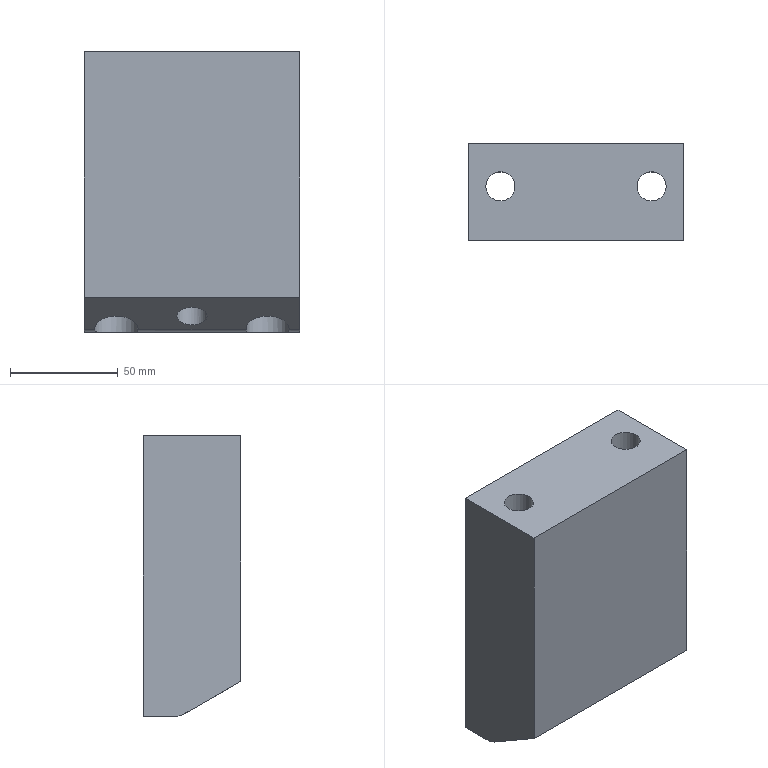Part | STEP file | lll_id3694_x_t | 1 solid | 20 faces | box 100 x 45 x 130 mm | volume 491265 mm3 | plane 10 | cylinder 9 | cone 1 | commonest cylinder face diameters 20 x3 13.509 x2 20.008 x2 10.505 x1 14 x1
STEP:
#1=CARTESIAN_POINT('',(2964.747,-53.5,17.5));
#2=VERTEX_POINT('',#1);
#3=CARTESIAN_POINT('',(2970.,-53.5,17.5));
#4=DIRECTION('',(0.,0.,-1.));
#5=DIRECTION('',(-1.,0.,0.));
#6=AXIS2_PLACEMENT_3D('',#3,#4,#5);
#7=CIRCLE('',#6,5.253);
#8=EDGE_CURVE('',#2,#2,#7,.T.);
#9=ORIENTED_EDGE('',*,*,#8,.F.);
#10=EDGE_LOOP('',(#9));
#11=FACE_BOUND('',#10,.T.);
#12=CARTESIAN_POINT('',(2963.,-53.5,17.5));
#13=VERTEX_POINT('',#12);
#14=CARTESIAN_POINT('',(2970.,-53.5,17.5));
#15=DIRECTION('',(0.,0.,-1.));
#16=DIRECTION('',(-1.,0.,0.));
#17=AXIS2_PLACEMENT_3D('',#14,#15,#16);
#18=CIRCLE('',#17,7.);
#19=EDGE_CURVE('',#13,#13,#18,.T.);
#20=ORIENTED_EDGE('',*,*,#19,.T.);
#21=EDGE_LOOP('',(#20));
#22=FACE_BOUND('',#21,.T.);
#23=CARTESIAN_POINT('',(2970.,-53.5,17.5));
#24=DIRECTION('',(0.,0.,1.));
#25=DIRECTION('',(-1.,0.,0.));
#26=AXIS2_PLACEMENT_3D('',#23,#24,#25);
#27=PLANE('',#26);
#28=ADVANCED_FACE('',(#11,#22),#27,.F.);
#29=CARTESIAN_POINT('',(2941.755,-43.5,92.5));
#30=VERTEX_POINT('',#29);
#31=CARTESIAN_POINT('',(2935.,-43.5,92.5));
#32=DIRECTION('',(0.,0.,1.));
#33=DIRECTION('',(1.,0.,0.));
#34=AXIS2_PLACEMENT_3D('',#31,#32,#33);
#35=CIRCLE('',#34,6.755);
#36=EDGE_CURVE('',#30,#30,#35,.T.);
#37=ORIENTED_EDGE('',*,*,#36,.F.);
#38=EDGE_LOOP('',(#37));
#39=FACE_BOUND('',#38,.T.);
#40=CARTESIAN_POINT('',(2941.755,-43.5,132.5));
#41=VERTEX_POINT('',#40);
#42=CARTESIAN_POINT('',(2935.,-43.5,132.5));
#43=DIRECTION('',(0.,0.,-1.));
#44=DIRECTION('',(1.,0.,0.));
#45=AXIS2_PLACEMENT_3D('',#42,#43,#44);
#46=CIRCLE('',#45,6.755);
#47=EDGE_CURVE('',#41,#41,#46,.T.);
#48=ORIENTED_EDGE('',*,*,#47,.F.);
#49=EDGE_LOOP('',(#48));
#50=FACE_BOUND('',#49,.T.);
#51=CARTESIAN_POINT('',(2935.,-43.5,2.5));
#52=DIRECTION('',(0.,0.,1.));
#53=DIRECTION('',(1.,0.,0.));
#54=AXIS2_PLACEMENT_3D('',#51,#52,#53);
#55=CYLINDRICAL_SURFACE('',#54,6.755);
#56=ADVANCED_FACE('',(#39,#50),#55,.F.);
#57=CARTESIAN_POINT('',(3011.755,-43.5,92.5));
#58=VERTEX_POINT('',#57);
#59=CARTESIAN_POINT('',(3005.,-43.5,92.5));
#60=DIRECTION('',(0.,0.,-1.));
#61=DIRECTION('',(1.,0.,0.));
#62=AXIS2_PLACEMENT_3D('',#59,#60,#61);
#63=CIRCLE('',#62,6.755);
#64=EDGE_CURVE('',#58,#58,#63,.T.);
#65=ORIENTED_EDGE('',*,*,#64,.T.);
#66=EDGE_LOOP('',(#65));
#67=FACE_BOUND('',#66,.T.);
#68=CARTESIAN_POINT('',(3011.755,-43.5,132.5));
#69=VERTEX_POINT('',#68);
#70=CARTESIAN_POINT('',(3005.,-43.5,132.5));
#71=DIRECTION('',(0.,0.,-1.));
#72=DIRECTION('',(1.,0.,0.));
#73=AXIS2_PLACEMENT_3D('',#70,#71,#72);
#74=CIRCLE('',#73,6.755);
#75=EDGE_CURVE('',#69,#69,#74,.T.);
#76=ORIENTED_EDGE('',*,*,#75,.F.);
#77=EDGE_LOOP('',(#76));
#78=FACE_BOUND('',#77,.T.);
#79=CARTESIAN_POINT('',(3005.,-43.5,2.5));
#80=DIRECTION('',(0.,0.,1.));
#81=DIRECTION('',(-1.,0.,0.));
#82=AXIS2_PLACEMENT_3D('',#79,#80,#81);
#83=CYLINDRICAL_SURFACE('',#82,6.755);
#84=ADVANCED_FACE('',(#67,#78),#83,.F.);
#85=CARTESIAN_POINT('',(2925.025,-42.737,3.84));
#86=VERTEX_POINT('',#85);
#87=CARTESIAN_POINT('',(2920.,-42.737,3.84));
#88=VERTEX_POINT('',#87);
#89=CARTESIAN_POINT('',(2935.,-42.737,3.84));
#90=DIRECTION('',(-1.,0.,0.));
#91=VECTOR('',#90,1.);
#92=LINE('',#89,#91);
#93=EDGE_CURVE('',#86,#88,#92,.T.);
#94=ORIENTED_EDGE('',*,*,#93,.T.);
#95=CARTESIAN_POINT('',(2920.,-37.737,2.5));
#96=VERTEX_POINT('',#95);
#97=CARTESIAN_POINT('',(2920.,-37.737,12.5));
#98=DIRECTION('',(-1.,0.,0.));
#99=DIRECTION('',(0.,0.,-1.));
#100=AXIS2_PLACEMENT_3D('',#97,#98,#99);
#101=CIRCLE('',#100,10.);
#102=EDGE_CURVE('',#96,#88,#101,.T.);
#103=ORIENTED_EDGE('',*,*,#102,.F.);
#104=CARTESIAN_POINT('',(2926.823,-37.737,2.5));
#105=VERTEX_POINT('',#104);
#106=CARTESIAN_POINT('',(2935.,-37.737,2.5));
#107=DIRECTION('',(-1.,0.,0.));
#108=VECTOR('',#107,1.);
#109=LINE('',#106,#108);
#110=EDGE_CURVE('',#105,#96,#109,.T.);
#111=ORIENTED_EDGE('',*,*,#110,.F.);
#112=CARTESIAN_POINT('',(2925.025,-42.737,3.84));
#113=CARTESIAN_POINT('',(2925.15,-41.107,2.899));
#114=CARTESIAN_POINT('',(2925.737,-39.278,2.5));
#115=CARTESIAN_POINT('',(2926.823,-37.737,2.5));
#116=B_SPLINE_CURVE_WITH_KNOTS('',3,(#112,#113,#114,#115),.UNSPECIFIED.,.F.,.F.,(4,4),(0.,1.),.UNSPECIFIED.);
#117=EDGE_CURVE('',#86,#105,#116,.T.);
#118=ORIENTED_EDGE('',*,*,#117,.F.);
#119=EDGE_LOOP('',(#94,#103,#111,#118));
#120=FACE_OUTER_BOUND('',#119,.T.);
#121=CARTESIAN_POINT('',(2935.,-37.737,12.5));
#122=DIRECTION('',(-1.,0.,0.));
#123=DIRECTION('',(0.,0.,-1.));
#124=AXIS2_PLACEMENT_3D('',#121,#122,#123);
#125=CYLINDRICAL_SURFACE('',#124,10.);
#126=ADVANCED_FACE('',(#120),#125,.T.);
#127=CARTESIAN_POINT('',(3020.,-37.737,2.5));
#128=VERTEX_POINT('',#127);
#129=CARTESIAN_POINT('',(3013.177,-37.737,2.5));
#130=VERTEX_POINT('',#129);
#131=CARTESIAN_POINT('',(2935.,-37.737,2.5));
#132=DIRECTION('',(-1.,0.,0.));
#133=VECTOR('',#132,1.);
#134=LINE('',#131,#133);
#135=EDGE_CURVE('',#128,#130,#134,.T.);
#136=ORIENTED_EDGE('',*,*,#135,.F.);
#137=CARTESIAN_POINT('',(3020.,-42.737,3.84));
#138=VERTEX_POINT('',#137);
#139=CARTESIAN_POINT('',(3020.,-37.737,12.5));
#140=DIRECTION('',(-1.,0.,0.));
#141=DIRECTION('',(0.,0.,1.));
#142=AXIS2_PLACEMENT_3D('',#139,#140,#141);
#143=CIRCLE('',#142,10.);
#144=EDGE_CURVE('',#128,#138,#143,.T.);
#145=ORIENTED_EDGE('',*,*,#144,.T.);
#146=CARTESIAN_POINT('',(3014.975,-42.737,3.84));
#147=VERTEX_POINT('',#146);
#148=CARTESIAN_POINT('',(2935.,-42.737,3.84));
#149=DIRECTION('',(-1.,0.,0.));
#150=VECTOR('',#149,1.);
#151=LINE('',#148,#150);
#152=EDGE_CURVE('',#138,#147,#151,.T.);
#153=ORIENTED_EDGE('',*,*,#152,.T.);
#154=CARTESIAN_POINT('',(3013.177,-37.737,2.5));
#155=CARTESIAN_POINT('',(3014.263,-39.277,2.5));
#156=CARTESIAN_POINT('',(3014.85,-41.107,2.899));
#157=CARTESIAN_POINT('',(3014.975,-42.737,3.84));
#158=B_SPLINE_CURVE_WITH_KNOTS('',3,(#154,#155,#156,#157),.UNSPECIFIED.,.F.,.F.,(4,4),(0.,1.),.UNSPECIFIED.);
#159=EDGE_CURVE('',#130,#147,#158,.T.);
#160=ORIENTED_EDGE('',*,*,#159,.F.);
#161=EDGE_LOOP('',(#136,#145,#153,#160));
#162=FACE_OUTER_BOUND('',#161,.T.);
#163=CARTESIAN_POINT('',(2935.,-37.737,12.5));
#164=DIRECTION('',(-1.,0.,0.));
#165=DIRECTION('',(0.,0.,-1.));
#166=AXIS2_PLACEMENT_3D('',#163,#164,#165);
#167=CYLINDRICAL_SURFACE('',#166,10.);
#168=ADVANCED_FACE('',(#162),#167,.T.);
#169=ORIENTED_EDGE('',*,*,#110,.T.);
#170=CARTESIAN_POINT('',(2920.,-23.5,2.5));
#171=VERTEX_POINT('',#170);
#172=CARTESIAN_POINT('',(2920.,-30.25,2.5));
#173=DIRECTION('',(0.,-1.,0.));
#174=VECTOR('',#173,1.);
#175=LINE('',#172,#174);
#176=EDGE_CURVE('',#171,#96,#175,.T.);
#177=ORIENTED_EDGE('',*,*,#176,.F.);
#178=CARTESIAN_POINT('',(3020.,-23.5,2.5));
#179=VERTEX_POINT('',#178);
#180=CARTESIAN_POINT('',(2935.,-23.5,2.5));
#181=DIRECTION('',(-1.,0.,0.));
#182=VECTOR('',#181,1.);
#183=LINE('',#180,#182);
#184=EDGE_CURVE('',#179,#171,#183,.T.);
#185=ORIENTED_EDGE('',*,*,#184,.F.);
#186=CARTESIAN_POINT('',(3020.,25.737,2.5));
#187=DIRECTION('',(0.,-1.,0.));
#188=VECTOR('',#187,1.);
#189=LINE('',#186,#188);
#190=EDGE_CURVE('',#179,#128,#189,.T.);
#191=ORIENTED_EDGE('',*,*,#190,.T.);
#192=ORIENTED_EDGE('',*,*,#135,.T.);
#193=CARTESIAN_POINT('',(2996.823,-37.737,2.5));
#194=VERTEX_POINT('',#193);
#195=CARTESIAN_POINT('',(3005.,-43.5,2.5));
#196=DIRECTION('',(0.,0.,-1.));
#197=DIRECTION('',(-1.,0.,0.));
#198=AXIS2_PLACEMENT_3D('',#195,#196,#197);
#199=CIRCLE('',#198,10.004);
#200=EDGE_CURVE('',#194,#130,#199,.T.);
#201=ORIENTED_EDGE('',*,*,#200,.F.);
#202=CARTESIAN_POINT('',(2943.177,-37.737,2.5));
#203=VERTEX_POINT('',#202);
#204=CARTESIAN_POINT('',(2935.,-37.737,2.5));
#205=DIRECTION('',(-1.,0.,0.));
#206=VECTOR('',#205,1.);
#207=LINE('',#204,#206);
#208=EDGE_CURVE('',#194,#203,#207,.T.);
#209=ORIENTED_EDGE('',*,*,#208,.T.);
#210=CARTESIAN_POINT('',(2935.,-43.5,2.5));
#211=DIRECTION('',(0.,0.,-1.));
#212=DIRECTION('',(-1.,0.,0.));
#213=AXIS2_PLACEMENT_3D('',#210,#211,#212);
#214=CIRCLE('',#213,10.004);
#215=EDGE_CURVE('',#105,#203,#214,.T.);
#216=ORIENTED_EDGE('',*,*,#215,.F.);
#217=EDGE_LOOP('',(#169,#177,#185,#191,#192,#201,#209,#216));
#218=FACE_OUTER_BOUND('',#217,.T.);
#219=CARTESIAN_POINT('',(2935.,25.737,2.5));
#220=DIRECTION('',(0.,0.,1.));
#221=DIRECTION('',(-1.,0.,0.));
#222=AXIS2_PLACEMENT_3D('',#219,#220,#221);
#223=PLANE('',#222);
#224=ADVANCED_FACE('',(#218),#223,.F.);
#225=ORIENTED_EDGE('',*,*,#47,.T.);
#226=EDGE_LOOP('',(#225));
#227=FACE_BOUND('',#226,.T.);
#228=ORIENTED_EDGE('',*,*,#75,.T.);
#229=EDGE_LOOP('',(#228));
#230=FACE_BOUND('',#229,.T.);
#231=CARTESIAN_POINT('',(3020.,-68.5,132.5));
#232=VERTEX_POINT('',#231);
#233=CARTESIAN_POINT('',(2920.,-68.5,132.5));
#234=VERTEX_POINT('',#233);
#235=CARTESIAN_POINT('',(2935.,-68.5,132.5));
#236=DIRECTION('',(-1.,0.,0.));
#237=VECTOR('',#236,1.);
#238=LINE('',#235,#237);
#239=EDGE_CURVE('',#232,#234,#238,.T.);
#240=ORIENTED_EDGE('',*,*,#239,.F.);
#241=CARTESIAN_POINT('',(3020.,-23.5,132.5));
#242=VERTEX_POINT('',#241);
#243=CARTESIAN_POINT('',(3020.,0.0001484,132.5));
#244=DIRECTION('',(0.,-1.,0.));
#245=VECTOR('',#244,1.);
#246=LINE('',#243,#245);
#247=EDGE_CURVE('',#242,#232,#246,.T.);
#248=ORIENTED_EDGE('',*,*,#247,.F.);
#249=CARTESIAN_POINT('',(2920.,-23.5,132.5));
#250=VERTEX_POINT('',#249);
#251=CARTESIAN_POINT('',(-2196.249,-23.5,132.5));
#252=DIRECTION('',(1.,0.,0.));
#253=VECTOR('',#252,1.);
#254=LINE('',#251,#253);
#255=EDGE_CURVE('',#250,#242,#254,.T.);
#256=ORIENTED_EDGE('',*,*,#255,.F.);
#257=CARTESIAN_POINT('',(2920.,-30.25,132.5));
#258=DIRECTION('',(0.,-1.,0.));
#259=VECTOR('',#258,1.);
#260=LINE('',#257,#259);
#261=EDGE_CURVE('',#250,#234,#260,.T.);
#262=ORIENTED_EDGE('',*,*,#261,.T.);
#263=EDGE_LOOP('',(#240,#248,#256,#262));
#264=FACE_BOUND('',#263,.T.);
#265=CARTESIAN_POINT('',(-2196.249,0.0001484,132.5));
#266=DIRECTION('',(0.,0.,-1.));
#267=DIRECTION('',(1.,0.,0.));
#268=AXIS2_PLACEMENT_3D('',#265,#266,#267);
#269=PLANE('',#268);
#270=ADVANCED_FACE('',(#227,#230,#264),#269,.F.);
#271=ORIENTED_EDGE('',*,*,#208,.F.);
#272=CARTESIAN_POINT('',(2995.025,-42.737,3.84));
#273=VERTEX_POINT('',#272);
#274=CARTESIAN_POINT('',(2995.025,-42.737,3.84));
#275=CARTESIAN_POINT('',(2995.15,-41.107,2.899));
#276=CARTESIAN_POINT('',(2995.737,-39.278,2.5));
#277=CARTESIAN_POINT('',(2996.823,-37.737,2.5));
#278=B_SPLINE_CURVE_WITH_KNOTS('',3,(#274,#275,#276,#277),.UNSPECIFIED.,.F.,.F.,(4,4),(0.,1.),.UNSPECIFIED.);
#279=EDGE_CURVE('',#273,#194,#278,.T.);
#280=ORIENTED_EDGE('',*,*,#279,.F.);
#281=CARTESIAN_POINT('',(2944.975,-42.737,3.84));
#282=VERTEX_POINT('',#281);
#283=CARTESIAN_POINT('',(2935.,-42.737,3.84));
#284=DIRECTION('',(-1.,0.,0.));
#285=VECTOR('',#284,1.);
#286=LINE('',#283,#285);
#287=EDGE_CURVE('',#273,#282,#286,.T.);
#288=ORIENTED_EDGE('',*,*,#287,.T.);
#289=CARTESIAN_POINT('',(2943.177,-37.737,2.5));
#290=CARTESIAN_POINT('',(2944.263,-39.277,2.5));
#291=CARTESIAN_POINT('',(2944.85,-41.107,2.899));
#292=CARTESIAN_POINT('',(2944.975,-42.737,3.84));
#293=B_SPLINE_CURVE_WITH_KNOTS('',3,(#289,#290,#291,#292),.UNSPECIFIED.,.F.,.F.,(4,4),(0.,1.),.UNSPECIFIED.);
#294=EDGE_CURVE('',#203,#282,#293,.T.);
#295=ORIENTED_EDGE('',*,*,#294,.F.);
#296=EDGE_LOOP('',(#271,#280,#288,#295));
#297=FACE_OUTER_BOUND('',#296,.T.);
#298=CARTESIAN_POINT('',(2935.,-37.737,12.5));
#299=DIRECTION('',(-1.,0.,0.));
#300=DIRECTION('',(0.,0.,-1.));
#301=AXIS2_PLACEMENT_3D('',#298,#299,#300);
#302=CYLINDRICAL_SURFACE('',#301,10.);
#303=ADVANCED_FACE('',(#297),#302,.T.);
#304=CARTESIAN_POINT('',(2970.,-60.5,14.095));
#305=VERTEX_POINT('',#304);
#306=CARTESIAN_POINT('',(2970.,-53.5,10.054));
#307=DIRECTION('',(0.,-0.5,-0.866));
#308=DIRECTION('',(0.,-0.866,0.5));
#309=AXIS2_PLACEMENT_3D('',#306,#307,#308);
#310=ELLIPSE('',#309,8.083,7.);
#311=EDGE_CURVE('',#305,#305,#310,.T.);
#312=ORIENTED_EDGE('',*,*,#311,.F.);
#313=EDGE_LOOP('',(#312));
#314=FACE_BOUND('',#313,.T.);
#315=ORIENTED_EDGE('',*,*,#287,.F.);
#316=CARTESIAN_POINT('',(3005.,-43.5,4.28));
#317=DIRECTION('',(0.,-0.5,-0.866));
#318=DIRECTION('',(0.,-0.866,0.5));
#319=AXIS2_PLACEMENT_3D('',#316,#317,#318);
#320=ELLIPSE('',#319,11.552,10.004);
#321=EDGE_CURVE('',#147,#273,#320,.T.);
#322=ORIENTED_EDGE('',*,*,#321,.F.);
#323=ORIENTED_EDGE('',*,*,#152,.F.);
#324=CARTESIAN_POINT('',(3020.,-68.5,18.714));
#325=VERTEX_POINT('',#324);
#326=CARTESIAN_POINT('',(3020.,-42.737,3.84));
#327=DIRECTION('',(0.,-0.866,0.5));
#328=VECTOR('',#327,1.);
#329=LINE('',#326,#328);
#330=EDGE_CURVE('',#138,#325,#329,.T.);
#331=ORIENTED_EDGE('',*,*,#330,.T.);
#332=CARTESIAN_POINT('',(2920.,-68.5,18.714));
#333=VERTEX_POINT('',#332);
#334=CARTESIAN_POINT('',(2935.,-68.5,18.714));
#335=DIRECTION('',(1.,0.,0.));
#336=VECTOR('',#335,1.);
#337=LINE('',#334,#336);
#338=EDGE_CURVE('',#333,#325,#337,.T.);
#339=ORIENTED_EDGE('',*,*,#338,.F.);
#340=CARTESIAN_POINT('',(2920.,-42.737,3.84));
#341=DIRECTION('',(0.,0.866,-0.5));
#342=VECTOR('',#341,1.);
#343=LINE('',#340,#342);
#344=EDGE_CURVE('',#333,#88,#343,.T.);
#345=ORIENTED_EDGE('',*,*,#344,.T.);
#346=ORIENTED_EDGE('',*,*,#93,.F.);
#347=CARTESIAN_POINT('',(2935.,-43.5,4.28));
#348=DIRECTION('',(0.,-0.5,-0.866));
#349=DIRECTION('',(0.,-0.866,0.5));
#350=AXIS2_PLACEMENT_3D('',#347,#348,#349);
#351=ELLIPSE('',#350,11.552,10.004);
#352=EDGE_CURVE('',#282,#86,#351,.T.);
#353=ORIENTED_EDGE('',*,*,#352,.F.);
#354=EDGE_LOOP('',(#315,#322,#323,#331,#339,#345,#346,#353));
#355=FACE_BOUND('',#354,.T.);
#356=CARTESIAN_POINT('',(2935.,-42.737,3.84));
#357=DIRECTION('',(0.,0.5,0.866));
#358=DIRECTION('',(0.,-0.866,0.5));
#359=AXIS2_PLACEMENT_3D('',#356,#357,#358);
#360=PLANE('',#359);
#361=ADVANCED_FACE('',(#314,#355),#360,.F.);
#362=ORIENTED_EDGE('',*,*,#255,.T.);
#363=CARTESIAN_POINT('',(3020.,-23.5,22.5));
#364=DIRECTION('',(0.,0.,-1.));
#365=VECTOR('',#364,1.);
#366=LINE('',#363,#365);
#367=EDGE_CURVE('',#242,#179,#366,.T.);
#368=ORIENTED_EDGE('',*,*,#367,.T.);
#369=ORIENTED_EDGE('',*,*,#184,.T.);
#370=CARTESIAN_POINT('',(2920.,-23.5,11.25));
#371=DIRECTION('',(0.,0.,1.));
#372=VECTOR('',#371,1.);
#373=LINE('',#370,#372);
#374=EDGE_CURVE('',#171,#250,#373,.T.);
#375=ORIENTED_EDGE('',*,*,#374,.T.);
#376=EDGE_LOOP('',(#362,#368,#369,#375));
#377=FACE_OUTER_BOUND('',#376,.T.);
#378=CARTESIAN_POINT('',(2935.,-23.5,62.5));
#379=DIRECTION('',(0.,1.,0.));
#380=DIRECTION('',(0.,0.,1.));
#381=AXIS2_PLACEMENT_3D('',#378,#379,#380);
#382=PLANE('',#381);
#383=ADVANCED_FACE('',(#377),#382,.T.);
#384=CARTESIAN_POINT('',(2920.,-68.5,62.5));
#385=DIRECTION('',(0.,0.,-1.));
#386=VECTOR('',#385,1.);
#387=LINE('',#384,#386);
#388=EDGE_CURVE('',#234,#333,#387,.T.);
#389=ORIENTED_EDGE('',*,*,#388,.T.);
#390=ORIENTED_EDGE('',*,*,#338,.T.);
#391=CARTESIAN_POINT('',(3020.,-68.5,22.5));
#392=DIRECTION('',(0.,0.,-1.));
#393=VECTOR('',#392,1.);
#394=LINE('',#391,#393);
#395=EDGE_CURVE('',#232,#325,#394,.T.);
#396=ORIENTED_EDGE('',*,*,#395,.F.);
#397=ORIENTED_EDGE('',*,*,#239,.T.);
#398=EDGE_LOOP('',(#389,#390,#396,#397));
#399=FACE_OUTER_BOUND('',#398,.T.);
#400=CARTESIAN_POINT('',(2935.,-68.5,62.5));
#401=DIRECTION('',(0.,1.,0.));
#402=DIRECTION('',(0.,0.,1.));
#403=AXIS2_PLACEMENT_3D('',#400,#401,#402);
#404=PLANE('',#403);
#405=ADVANCED_FACE('',(#399),#404,.F.);
#406=ORIENTED_EDGE('',*,*,#395,.T.);
#407=ORIENTED_EDGE('',*,*,#330,.F.);
#408=ORIENTED_EDGE('',*,*,#144,.F.);
#409=ORIENTED_EDGE('',*,*,#190,.F.);
#410=ORIENTED_EDGE('',*,*,#367,.F.);
#411=ORIENTED_EDGE('',*,*,#247,.T.);
#412=EDGE_LOOP('',(#406,#407,#408,#409,#410,#411));
#413=FACE_OUTER_BOUND('',#412,.T.);
#414=CARTESIAN_POINT('',(3020.,-27.737,22.5));
#415=DIRECTION('',(1.,0.,0.));
#416=DIRECTION('',(0.,0.,1.));
#417=AXIS2_PLACEMENT_3D('',#414,#415,#416);
#418=PLANE('',#417);
#419=ADVANCED_FACE('',(#413),#418,.T.);
#420=ORIENTED_EDGE('',*,*,#374,.F.);
#421=ORIENTED_EDGE('',*,*,#176,.T.);
#422=ORIENTED_EDGE('',*,*,#102,.T.);
#423=ORIENTED_EDGE('',*,*,#344,.F.);
#424=ORIENTED_EDGE('',*,*,#388,.F.);
#425=ORIENTED_EDGE('',*,*,#261,.F.);
#426=EDGE_LOOP('',(#420,#421,#422,#423,#424,#425));
#427=FACE_OUTER_BOUND('',#426,.T.);
#428=CARTESIAN_POINT('',(2920.,-30.25,11.25));
#429=DIRECTION('',(-1.,0.,0.));
#430=DIRECTION('',(0.,0.,-1.));
#431=AXIS2_PLACEMENT_3D('',#428,#429,#430);
#432=PLANE('',#431);
#433=ADVANCED_FACE('',(#427),#432,.T.);
#434=CARTESIAN_POINT('',(3015.004,-43.5,92.5));
#435=VERTEX_POINT('',#434);
#436=CARTESIAN_POINT('',(3005.,-43.5,92.5));
#437=DIRECTION('',(0.,0.,-1.));
#438=DIRECTION('',(1.,0.,0.));
#439=AXIS2_PLACEMENT_3D('',#436,#437,#438);
#440=CIRCLE('',#439,10.004);
#441=EDGE_CURVE('',#435,#435,#440,.T.);
#442=ORIENTED_EDGE('',*,*,#441,.F.);
#443=EDGE_LOOP('',(#442));
#444=FACE_BOUND('',#443,.T.);
#445=ORIENTED_EDGE('',*,*,#279,.T.);
#446=ORIENTED_EDGE('',*,*,#200,.T.);
#447=ORIENTED_EDGE('',*,*,#159,.T.);
#448=ORIENTED_EDGE('',*,*,#321,.T.);
#449=EDGE_LOOP('',(#445,#446,#447,#448));
#450=FACE_BOUND('',#449,.T.);
#451=CARTESIAN_POINT('',(3005.,-43.5,2.5));
#452=DIRECTION('',(0.,0.,1.));
#453=DIRECTION('',(-1.,0.,0.));
#454=AXIS2_PLACEMENT_3D('',#451,#452,#453);
#455=CYLINDRICAL_SURFACE('',#454,10.004);
#456=ADVANCED_FACE('',(#444,#450),#455,.F.);
#457=ORIENTED_EDGE('',*,*,#64,.F.);
#458=EDGE_LOOP('',(#457));
#459=FACE_BOUND('',#458,.T.);
#460=ORIENTED_EDGE('',*,*,#441,.T.);
#461=EDGE_LOOP('',(#460));
#462=FACE_BOUND('',#461,.T.);
#463=CARTESIAN_POINT('',(-2196.249,-5.,92.5));
#464=DIRECTION('',(0.,0.,-1.));
#465=DIRECTION('',(1.,0.,0.));
#466=AXIS2_PLACEMENT_3D('',#463,#464,#465);
#467=PLANE('',#466);
#468=ADVANCED_FACE('',(#459,#462),#467,.T.);
#469=CARTESIAN_POINT('',(2945.004,-43.5,92.5));
#470=VERTEX_POINT('',#469);
#471=CARTESIAN_POINT('',(2935.,-43.5,92.5));
#472=DIRECTION('',(0.,0.,1.));
#473=DIRECTION('',(1.,0.,0.));
#474=AXIS2_PLACEMENT_3D('',#471,#472,#473);
#475=CIRCLE('',#474,10.004);
#476=EDGE_CURVE('',#470,#470,#475,.T.);
#477=ORIENTED_EDGE('',*,*,#476,.T.);
#478=EDGE_LOOP('',(#477));
#479=FACE_BOUND('',#478,.T.);
#480=ORIENTED_EDGE('',*,*,#117,.T.);
#481=ORIENTED_EDGE('',*,*,#215,.T.);
#482=ORIENTED_EDGE('',*,*,#294,.T.);
#483=ORIENTED_EDGE('',*,*,#352,.T.);
#484=EDGE_LOOP('',(#480,#481,#482,#483));
#485=FACE_BOUND('',#484,.T.);
#486=CARTESIAN_POINT('',(2935.,-43.5,2.5));
#487=DIRECTION('',(0.,0.,1.));
#488=DIRECTION('',(1.,0.,0.));
#489=AXIS2_PLACEMENT_3D('',#486,#487,#488);
#490=CYLINDRICAL_SURFACE('',#489,10.004);
#491=ADVANCED_FACE('',(#479,#485),#490,.F.);
#492=ORIENTED_EDGE('',*,*,#36,.T.);
#493=EDGE_LOOP('',(#492));
#494=FACE_BOUND('',#493,.T.);
#495=ORIENTED_EDGE('',*,*,#476,.F.);
#496=EDGE_LOOP('',(#495));
#497=FACE_BOUND('',#496,.T.);
#498=CARTESIAN_POINT('',(-2196.249,-5.,92.5));
#499=DIRECTION('',(0.,0.,-1.));
#500=DIRECTION('',(1.,0.,0.));
#501=AXIS2_PLACEMENT_3D('',#498,#499,#500);
#502=PLANE('',#501);
#503=ADVANCED_FACE('',(#494,#497),#502,.T.);
#504=ORIENTED_EDGE('',*,*,#19,.F.);
#505=EDGE_LOOP('',(#504));
#506=FACE_BOUND('',#505,.T.);
#507=ORIENTED_EDGE('',*,*,#311,.T.);
#508=EDGE_LOOP('',(#507));
#509=FACE_BOUND('',#508,.T.);
#510=CARTESIAN_POINT('',(2970.,-53.5,2.5));
#511=DIRECTION('',(0.,0.,1.));
#512=DIRECTION('',(-1.,0.,0.));
#513=AXIS2_PLACEMENT_3D('',#510,#511,#512);
#514=CYLINDRICAL_SURFACE('',#513,7.);
#515=ADVANCED_FACE('',(#506,#509),#514,.F.);
#516=CARTESIAN_POINT('',(2964.747,-53.5,52.254));
#517=VERTEX_POINT('',#516);
#518=CARTESIAN_POINT('',(2970.,-53.5,52.254));
#519=DIRECTION('',(0.,0.,-1.));
#520=DIRECTION('',(-1.,0.,0.));
#521=AXIS2_PLACEMENT_3D('',#518,#519,#520);
#522=CIRCLE('',#521,5.253);
#523=EDGE_CURVE('',#517,#517,#522,.T.);
#524=ORIENTED_EDGE('',*,*,#523,.F.);
#525=EDGE_LOOP('',(#524));
#526=FACE_BOUND('',#525,.T.);
#527=ORIENTED_EDGE('',*,*,#8,.T.);
#528=EDGE_LOOP('',(#527));
#529=FACE_BOUND('',#528,.T.);
#530=CARTESIAN_POINT('',(2970.,-53.5,17.5));
#531=DIRECTION('',(0.,0.,1.));
#532=DIRECTION('',(-1.,0.,0.));
#533=AXIS2_PLACEMENT_3D('',#530,#531,#532);
#534=CYLINDRICAL_SURFACE('',#533,5.253);
#535=ADVANCED_FACE('',(#526,#529),#534,.F.);
#536=CARTESIAN_POINT('',(2970.,-53.5,57.506));
#537=VERTEX_POINT('',#536);
#538=VERTEX_LOOP('',#537);
#539=FACE_BOUND('',#538,.T.);
#540=ORIENTED_EDGE('',*,*,#523,.T.);
#541=EDGE_LOOP('',(#540));
#542=FACE_BOUND('',#541,.T.);
#543=CARTESIAN_POINT('',(2970.,-53.5,52.254));
#544=DIRECTION('',(0.,0.,-1.));
#545=DIRECTION('',(1.,0.,0.));
#546=AXIS2_PLACEMENT_3D('',#543,#544,#545);
#547=CONICAL_SURFACE('',#546,5.253,45.);
#548=ADVANCED_FACE('',(#539,#542),#547,.F.);
#549=CLOSED_SHELL('',(#28,#56,#84,#126,#168,#224,#270,#303,#361,#383,#405,#419,#433,#456,#468,#491,#503,#515,#535,#548));
#550=MANIFOLD_SOLID_BREP('',#549);
#551=(LENGTH_UNIT()NAMED_UNIT(*)SI_UNIT(.MILLI.,.METRE.));
#552=UNCERTAINTY_MEASURE_WITH_UNIT(LENGTH_MEASURE(0.0508),#551,'','');
#553=(NAMED_UNIT(*)PLANE_ANGLE_UNIT()SI_UNIT($,.RADIAN.));
#554=PLANE_ANGLE_MEASURE_WITH_UNIT(PLANE_ANGLE_MEASURE(0.01745),#553);
#555=DIMENSIONAL_EXPONENTS(0.,0.,0.,0.,0.,0.,0.);
#556=(CONVERSION_BASED_UNIT('DEGREE',#554)NAMED_UNIT(#555)PLANE_ANGLE_UNIT());
#557=(NAMED_UNIT(*)SI_UNIT($,.STERADIAN.)SOLID_ANGLE_UNIT());
#558=(GEOMETRIC_REPRESENTATION_CONTEXT(3)GLOBAL_UNCERTAINTY_ASSIGNED_CONTEXT((#552))GLOBAL_UNIT_ASSIGNED_CONTEXT((#551,#556,#557))REPRESENTATION_CONTEXT('',''));
#559=ADVANCED_BREP_SHAPE_REPRESENTATION('',(#550),#558);